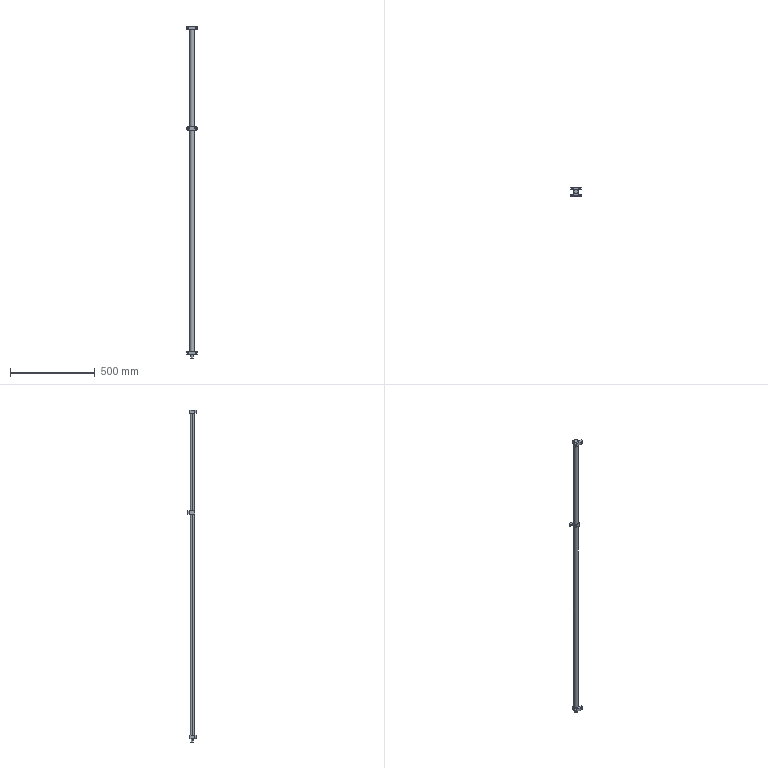Part | STEP file | Lead screw mount | 4 solids | 91 faces | box 60 x 50 x 1962 mm | volume 1004737 mm3 | plane 57 | cylinder 34 | commonest cylinder face diameters 6.6 x12 11 x12 25 x6 16 x2 24.9 x2